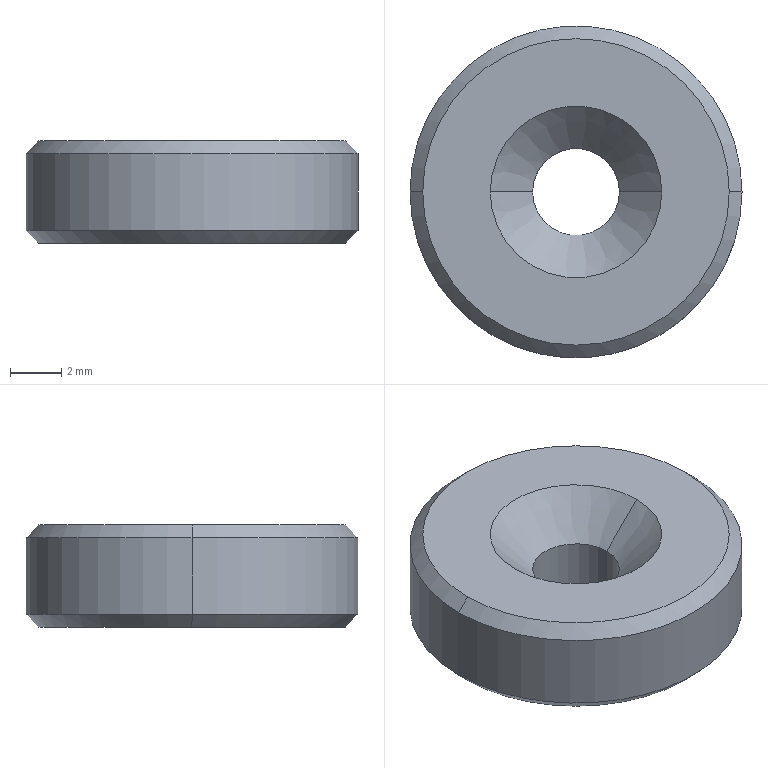Part | STEP file | 10000020551swp000-1 | 1 solid | 12 faces | box 13 x 13 x 4 mm | volume 465.157 mm3 | cone 6 | cylinder 4 | plane 2 | commonest cylinder face diameters 3.4 x2 13 x2
STEP:
#1=CARTESIAN_POINT('',(6.,0.,4.));
#2=VERTEX_POINT('',#1);
#3=CARTESIAN_POINT('',(-6.,0.,4.));
#4=VERTEX_POINT('',#3);
#5=CARTESIAN_POINT('',(0.,0.,4.));
#6=DIRECTION('',(0.,0.,1.));
#7=DIRECTION('',(1.,0.,0.));
#8=AXIS2_PLACEMENT_3D('',#5,#6,#7);
#9=CIRCLE('',#8,6.);
#10=EDGE_CURVE('',#2,#4,#9,.T.);
#11=ORIENTED_EDGE('',*,*,#10,.F.);
#12=CARTESIAN_POINT('',(6.5,0.,3.5));
#13=VERTEX_POINT('',#12);
#14=CARTESIAN_POINT('',(6.,0.,4.));
#15=DIRECTION('',(0.7071,0.,-0.7071));
#16=VECTOR('',#15,1000.);
#17=LINE('',#14,#16);
#18=EDGE_CURVE('',#2,#13,#17,.T.);
#19=ORIENTED_EDGE('',*,*,#18,.T.);
#20=CARTESIAN_POINT('',(-6.5,0.,3.5));
#21=VERTEX_POINT('',#20);
#22=CARTESIAN_POINT('',(0.,0.,3.5));
#23=DIRECTION('',(0.,0.,-1.));
#24=DIRECTION('',(1.,0.,0.));
#25=AXIS2_PLACEMENT_3D('',#22,#23,#24);
#26=CIRCLE('',#25,6.5);
#27=EDGE_CURVE('',#21,#13,#26,.T.);
#28=ORIENTED_EDGE('',*,*,#27,.F.);
#29=CARTESIAN_POINT('',(-6.,0.,4.));
#30=DIRECTION('',(-0.7071,0.,-0.7071));
#31=VECTOR('',#30,1000.);
#32=LINE('',#29,#31);
#33=EDGE_CURVE('',#4,#21,#32,.T.);
#34=ORIENTED_EDGE('',*,*,#33,.F.);
#35=EDGE_LOOP('',(#11,#19,#28,#34));
#36=FACE_OUTER_BOUND('',#35,.T.);
#37=CARTESIAN_POINT('',(0.,0.,4.));
#38=DIRECTION('',(0.,0.,-1.));
#39=DIRECTION('',(-1.,0.,0.));
#40=AXIS2_PLACEMENT_3D('',#37,#38,#39);
#41=CONICAL_SURFACE('',#40,6.,0.7854);
#42=ADVANCED_FACE('',(#36),#41,.T.);
#43=CARTESIAN_POINT('',(-6.,0.,0.));
#44=VERTEX_POINT('',#43);
#45=CARTESIAN_POINT('',(6.,0.,0.));
#46=VERTEX_POINT('',#45);
#47=CARTESIAN_POINT('',(0.,0.,0.));
#48=DIRECTION('',(0.,0.,-1.));
#49=DIRECTION('',(1.,0.,0.));
#50=AXIS2_PLACEMENT_3D('',#47,#48,#49);
#51=CIRCLE('',#50,6.);
#52=EDGE_CURVE('',#44,#46,#51,.T.);
#53=ORIENTED_EDGE('',*,*,#52,.F.);
#54=CARTESIAN_POINT('',(-6.5,0.,0.5));
#55=VERTEX_POINT('',#54);
#56=CARTESIAN_POINT('',(-6.5,0.,0.5));
#57=DIRECTION('',(-0.7071,0.,0.7071));
#58=VECTOR('',#57,1000.);
#59=LINE('',#56,#58);
#60=EDGE_CURVE('',#44,#55,#59,.T.);
#61=ORIENTED_EDGE('',*,*,#60,.T.);
#62=CARTESIAN_POINT('',(6.5,0.,0.5));
#63=VERTEX_POINT('',#62);
#64=CARTESIAN_POINT('',(0.,0.,0.5));
#65=DIRECTION('',(0.,0.,1.));
#66=DIRECTION('',(1.,0.,0.));
#67=AXIS2_PLACEMENT_3D('',#64,#65,#66);
#68=CIRCLE('',#67,6.5);
#69=EDGE_CURVE('',#63,#55,#68,.T.);
#70=ORIENTED_EDGE('',*,*,#69,.F.);
#71=CARTESIAN_POINT('',(6.5,0.,0.5));
#72=DIRECTION('',(0.7071,0.,0.7071));
#73=VECTOR('',#72,1000.);
#74=LINE('',#71,#73);
#75=EDGE_CURVE('',#46,#63,#74,.T.);
#76=ORIENTED_EDGE('',*,*,#75,.F.);
#77=EDGE_LOOP('',(#53,#61,#70,#76));
#78=FACE_OUTER_BOUND('',#77,.T.);
#79=CARTESIAN_POINT('',(0.,0.,0.5));
#80=DIRECTION('',(0.,0.,1.));
#81=DIRECTION('',(1.,0.,0.));
#82=AXIS2_PLACEMENT_3D('',#79,#80,#81);
#83=CONICAL_SURFACE('',#82,6.5,0.7854);
#84=ADVANCED_FACE('',(#78),#83,.T.);
#85=CARTESIAN_POINT('',(-1.7,0.,2.34));
#86=VERTEX_POINT('',#85);
#87=CARTESIAN_POINT('',(1.7,0.,2.34));
#88=VERTEX_POINT('',#87);
#89=CARTESIAN_POINT('',(0.,0.,2.34));
#90=DIRECTION('',(0.,0.,1.));
#91=DIRECTION('',(1.,0.,0.));
#92=AXIS2_PLACEMENT_3D('',#89,#90,#91);
#93=CIRCLE('',#92,1.7);
#94=EDGE_CURVE('',#86,#88,#93,.T.);
#95=ORIENTED_EDGE('',*,*,#94,.F.);
#96=CARTESIAN_POINT('',(-3.36,0.,4.));
#97=VERTEX_POINT('',#96);
#98=CARTESIAN_POINT('',(-3.36,0.,4.));
#99=DIRECTION('',(-0.7071,0.,0.7071));
#100=VECTOR('',#99,1000.);
#101=LINE('',#98,#100);
#102=EDGE_CURVE('',#86,#97,#101,.T.);
#103=ORIENTED_EDGE('',*,*,#102,.T.);
#104=CARTESIAN_POINT('',(3.36,0.,4.));
#105=VERTEX_POINT('',#104);
#106=CARTESIAN_POINT('',(0.,0.,4.));
#107=DIRECTION('',(0.,0.,1.));
#108=DIRECTION('',(1.,0.,0.));
#109=AXIS2_PLACEMENT_3D('',#106,#107,#108);
#110=CIRCLE('',#109,3.36);
#111=EDGE_CURVE('',#97,#105,#110,.T.);
#112=ORIENTED_EDGE('',*,*,#111,.T.);
#113=CARTESIAN_POINT('',(3.36,0.,4.));
#114=DIRECTION('',(0.7071,0.,0.7071));
#115=VECTOR('',#114,1000.);
#116=LINE('',#113,#115);
#117=EDGE_CURVE('',#88,#105,#116,.T.);
#118=ORIENTED_EDGE('',*,*,#117,.F.);
#119=EDGE_LOOP('',(#95,#103,#112,#118));
#120=FACE_OUTER_BOUND('',#119,.T.);
#121=CARTESIAN_POINT('',(0.,0.,4.));
#122=DIRECTION('',(0.,0.,1.));
#123=DIRECTION('',(1.,0.,0.));
#124=AXIS2_PLACEMENT_3D('',#121,#122,#123);
#125=CONICAL_SURFACE('',#124,3.36,0.7854);
#126=ADVANCED_FACE('',(#120),#125,.F.);
#127=CARTESIAN_POINT('',(-1.7,0.,0.));
#128=VERTEX_POINT('',#127);
#129=CARTESIAN_POINT('',(1.7,0.,0.));
#130=VERTEX_POINT('',#129);
#131=CARTESIAN_POINT('',(0.,0.,0.));
#132=DIRECTION('',(0.,0.,1.));
#133=DIRECTION('',(1.,0.,0.));
#134=AXIS2_PLACEMENT_3D('',#131,#132,#133);
#135=CIRCLE('',#134,1.7);
#136=EDGE_CURVE('',#128,#130,#135,.T.);
#137=ORIENTED_EDGE('',*,*,#136,.F.);
#138=CARTESIAN_POINT('',(-1.7,0.,4.));
#139=DIRECTION('',(0.,0.,1.));
#140=VECTOR('',#139,1000.);
#141=LINE('',#138,#140);
#142=EDGE_CURVE('',#128,#86,#141,.T.);
#143=ORIENTED_EDGE('',*,*,#142,.T.);
#144=ORIENTED_EDGE('',*,*,#94,.T.);
#145=CARTESIAN_POINT('',(1.7,0.,4.));
#146=DIRECTION('',(0.,0.,1.));
#147=VECTOR('',#146,1000.);
#148=LINE('',#145,#147);
#149=EDGE_CURVE('',#130,#88,#148,.T.);
#150=ORIENTED_EDGE('',*,*,#149,.F.);
#151=EDGE_LOOP('',(#137,#143,#144,#150));
#152=FACE_OUTER_BOUND('',#151,.T.);
#153=CARTESIAN_POINT('',(0.,0.,4.));
#154=DIRECTION('',(0.,0.,1.));
#155=DIRECTION('',(1.,0.,0.));
#156=AXIS2_PLACEMENT_3D('',#153,#154,#155);
#157=CYLINDRICAL_SURFACE('',#156,1.7);
#158=ADVANCED_FACE('',(#152),#157,.F.);
#159=ORIENTED_EDGE('',*,*,#27,.T.);
#160=CARTESIAN_POINT('',(6.5,0.,4.));
#161=DIRECTION('',(0.,0.,-1.));
#162=VECTOR('',#161,1000.);
#163=LINE('',#160,#162);
#164=EDGE_CURVE('',#13,#63,#163,.T.);
#165=ORIENTED_EDGE('',*,*,#164,.T.);
#166=ORIENTED_EDGE('',*,*,#69,.T.);
#167=CARTESIAN_POINT('',(-6.5,0.,4.));
#168=DIRECTION('',(0.,0.,-1.));
#169=VECTOR('',#168,1000.);
#170=LINE('',#167,#169);
#171=EDGE_CURVE('',#21,#55,#170,.T.);
#172=ORIENTED_EDGE('',*,*,#171,.F.);
#173=EDGE_LOOP('',(#159,#165,#166,#172));
#174=FACE_OUTER_BOUND('',#173,.T.);
#175=CARTESIAN_POINT('',(0.,0.,4.));
#176=DIRECTION('',(0.,0.,-1.));
#177=DIRECTION('',(-1.,0.,0.));
#178=AXIS2_PLACEMENT_3D('',#175,#176,#177);
#179=CYLINDRICAL_SURFACE('',#178,6.5);
#180=ADVANCED_FACE('',(#174),#179,.T.);
#181=ORIENTED_EDGE('',*,*,#164,.F.);
#182=CARTESIAN_POINT('',(0.,0.,3.5));
#183=DIRECTION('',(0.,0.,-1.));
#184=DIRECTION('',(1.,0.,0.));
#185=AXIS2_PLACEMENT_3D('',#182,#183,#184);
#186=CIRCLE('',#185,6.5);
#187=EDGE_CURVE('',#13,#21,#186,.T.);
#188=ORIENTED_EDGE('',*,*,#187,.T.);
#189=ORIENTED_EDGE('',*,*,#171,.T.);
#190=CARTESIAN_POINT('',(0.,0.,0.5));
#191=DIRECTION('',(0.,0.,1.));
#192=DIRECTION('',(1.,0.,0.));
#193=AXIS2_PLACEMENT_3D('',#190,#191,#192);
#194=CIRCLE('',#193,6.5);
#195=EDGE_CURVE('',#55,#63,#194,.T.);
#196=ORIENTED_EDGE('',*,*,#195,.T.);
#197=EDGE_LOOP('',(#181,#188,#189,#196));
#198=FACE_OUTER_BOUND('',#197,.T.);
#199=CARTESIAN_POINT('',(0.,0.,4.));
#200=DIRECTION('',(0.,0.,-1.));
#201=DIRECTION('',(-1.,0.,0.));
#202=AXIS2_PLACEMENT_3D('',#199,#200,#201);
#203=CYLINDRICAL_SURFACE('',#202,6.5);
#204=ADVANCED_FACE('',(#198),#203,.T.);
#205=CARTESIAN_POINT('',(0.,0.,4.));
#206=DIRECTION('',(0.,0.,1.));
#207=DIRECTION('',(1.,0.,0.));
#208=AXIS2_PLACEMENT_3D('',#205,#206,#207);
#209=CIRCLE('',#208,6.);
#210=EDGE_CURVE('',#4,#2,#209,.T.);
#211=ORIENTED_EDGE('',*,*,#210,.T.);
#212=ORIENTED_EDGE('',*,*,#10,.T.);
#213=EDGE_LOOP('',(#211,#212));
#214=FACE_OUTER_BOUND('',#213,.T.);
#215=CARTESIAN_POINT('',(0.,0.,4.));
#216=DIRECTION('',(0.,0.,1.));
#217=DIRECTION('',(1.,0.,0.));
#218=AXIS2_PLACEMENT_3D('',#215,#216,#217);
#219=CIRCLE('',#218,3.36);
#220=EDGE_CURVE('',#105,#97,#219,.T.);
#221=ORIENTED_EDGE('',*,*,#220,.F.);
#222=ORIENTED_EDGE('',*,*,#111,.F.);
#223=EDGE_LOOP('',(#221,#222));
#224=FACE_BOUND('',#223,.T.);
#225=CARTESIAN_POINT('',(0.,0.,4.));
#226=DIRECTION('',(0.,0.,1.));
#227=DIRECTION('',(1.,0.,0.));
#228=AXIS2_PLACEMENT_3D('',#225,#226,#227);
#229=PLANE('',#228);
#230=ADVANCED_FACE('',(#214,#224),#229,.T.);
#231=CARTESIAN_POINT('',(0.,0.,0.));
#232=DIRECTION('',(0.,0.,-1.));
#233=DIRECTION('',(1.,0.,0.));
#234=AXIS2_PLACEMENT_3D('',#231,#232,#233);
#235=CIRCLE('',#234,6.);
#236=EDGE_CURVE('',#46,#44,#235,.T.);
#237=ORIENTED_EDGE('',*,*,#236,.T.);
#238=ORIENTED_EDGE('',*,*,#52,.T.);
#239=EDGE_LOOP('',(#237,#238));
#240=FACE_OUTER_BOUND('',#239,.T.);
#241=CARTESIAN_POINT('',(0.,0.,0.));
#242=DIRECTION('',(0.,0.,1.));
#243=DIRECTION('',(1.,0.,0.));
#244=AXIS2_PLACEMENT_3D('',#241,#242,#243);
#245=CIRCLE('',#244,1.7);
#246=EDGE_CURVE('',#130,#128,#245,.T.);
#247=ORIENTED_EDGE('',*,*,#246,.T.);
#248=ORIENTED_EDGE('',*,*,#136,.T.);
#249=EDGE_LOOP('',(#247,#248));
#250=FACE_BOUND('',#249,.T.);
#251=CARTESIAN_POINT('',(0.,0.,0.));
#252=DIRECTION('',(0.,0.,1.));
#253=DIRECTION('',(1.,0.,0.));
#254=AXIS2_PLACEMENT_3D('',#251,#252,#253);
#255=PLANE('',#254);
#256=ADVANCED_FACE('',(#240,#250),#255,.F.);
#257=ORIENTED_EDGE('',*,*,#142,.F.);
#258=ORIENTED_EDGE('',*,*,#246,.F.);
#259=ORIENTED_EDGE('',*,*,#149,.T.);
#260=CARTESIAN_POINT('',(0.,0.,2.34));
#261=DIRECTION('',(0.,0.,1.));
#262=DIRECTION('',(1.,0.,0.));
#263=AXIS2_PLACEMENT_3D('',#260,#261,#262);
#264=CIRCLE('',#263,1.7);
#265=EDGE_CURVE('',#88,#86,#264,.T.);
#266=ORIENTED_EDGE('',*,*,#265,.T.);
#267=EDGE_LOOP('',(#257,#258,#259,#266));
#268=FACE_OUTER_BOUND('',#267,.T.);
#269=CARTESIAN_POINT('',(0.,0.,4.));
#270=DIRECTION('',(0.,0.,1.));
#271=DIRECTION('',(1.,0.,0.));
#272=AXIS2_PLACEMENT_3D('',#269,#270,#271);
#273=CYLINDRICAL_SURFACE('',#272,1.7);
#274=ADVANCED_FACE('',(#268),#273,.F.);
#275=ORIENTED_EDGE('',*,*,#102,.F.);
#276=ORIENTED_EDGE('',*,*,#265,.F.);
#277=ORIENTED_EDGE('',*,*,#117,.T.);
#278=ORIENTED_EDGE('',*,*,#220,.T.);
#279=EDGE_LOOP('',(#275,#276,#277,#278));
#280=FACE_OUTER_BOUND('',#279,.T.);
#281=CARTESIAN_POINT('',(0.,0.,4.));
#282=DIRECTION('',(0.,0.,1.));
#283=DIRECTION('',(1.,0.,0.));
#284=AXIS2_PLACEMENT_3D('',#281,#282,#283);
#285=CONICAL_SURFACE('',#284,3.36,0.7854);
#286=ADVANCED_FACE('',(#280),#285,.F.);
#287=ORIENTED_EDGE('',*,*,#60,.F.);
#288=ORIENTED_EDGE('',*,*,#236,.F.);
#289=ORIENTED_EDGE('',*,*,#75,.T.);
#290=ORIENTED_EDGE('',*,*,#195,.F.);
#291=EDGE_LOOP('',(#287,#288,#289,#290));
#292=FACE_OUTER_BOUND('',#291,.T.);
#293=CARTESIAN_POINT('',(0.,0.,0.5));
#294=DIRECTION('',(0.,0.,1.));
#295=DIRECTION('',(1.,0.,0.));
#296=AXIS2_PLACEMENT_3D('',#293,#294,#295);
#297=CONICAL_SURFACE('',#296,6.5,0.7854);
#298=ADVANCED_FACE('',(#292),#297,.T.);
#299=ORIENTED_EDGE('',*,*,#18,.F.);
#300=ORIENTED_EDGE('',*,*,#210,.F.);
#301=ORIENTED_EDGE('',*,*,#33,.T.);
#302=ORIENTED_EDGE('',*,*,#187,.F.);
#303=EDGE_LOOP('',(#299,#300,#301,#302));
#304=FACE_OUTER_BOUND('',#303,.T.);
#305=CARTESIAN_POINT('',(0.,0.,4.));
#306=DIRECTION('',(0.,0.,-1.));
#307=DIRECTION('',(-1.,0.,0.));
#308=AXIS2_PLACEMENT_3D('',#305,#306,#307);
#309=CONICAL_SURFACE('',#308,6.,0.7854);
#310=ADVANCED_FACE('',(#304),#309,.T.);
#311=CLOSED_SHELL('',(#42,#84,#126,#158,#180,#204,#230,#256,#274,#286,#298,#310));
#312=MANIFOLD_SOLID_BREP('',#311);
#313=CARTESIAN_POINT('',(0.,0.,0.));
#314=DIRECTION('',(0.,0.,1.));
#315=DIRECTION('',(1.,0.,0.));
#316=AXIS2_PLACEMENT_3D('',#313,#314,#315);
#317=(LENGTH_UNIT()NAMED_UNIT(*)SI_UNIT(.MILLI.,.METRE.));
#318=UNCERTAINTY_MEASURE_WITH_UNIT(LENGTH_MEASURE(0.00001),#317,'','');
#319=(NAMED_UNIT(*)PLANE_ANGLE_UNIT()SI_UNIT($,.RADIAN.));
#320=(NAMED_UNIT(*)SI_UNIT($,.STERADIAN.)SOLID_ANGLE_UNIT());
#321=(GEOMETRIC_REPRESENTATION_CONTEXT(3)GLOBAL_UNCERTAINTY_ASSIGNED_CONTEXT((#318))GLOBAL_UNIT_ASSIGNED_CONTEXT((#317,#319,#320))REPRESENTATION_CONTEXT('',''));
#322=ADVANCED_BREP_SHAPE_REPRESENTATION('',(#312,#316),#321);